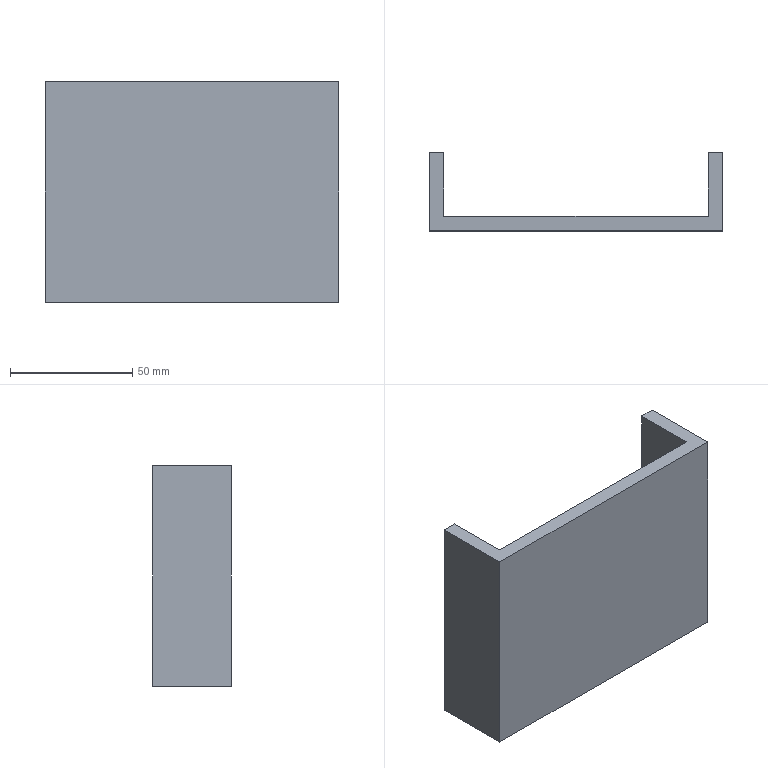Part | SolidWorks | features Extrusion 1 | 1 solid | 10 faces | box 120 x 32 x 90 mm | volume 92880 mm3 | plane 10
STEP:
#1=CARTESIAN_POINT('',(-60.,32.,45.));
#2=VERTEX_POINT('',#1);
#3=CARTESIAN_POINT('',(-60.,0.,45.));
#4=VERTEX_POINT('',#3);
#5=CARTESIAN_POINT('',(-60.,32.,45.));
#6=DIRECTION('',(0.,-1.,0.));
#7=VECTOR('',#6,1000.);
#8=LINE('',#5,#7);
#9=EDGE_CURVE('',#2,#4,#8,.T.);
#10=ORIENTED_EDGE('',*,*,#9,.F.);
#11=CARTESIAN_POINT('',(-60.,32.,-45.));
#12=VERTEX_POINT('',#11);
#13=CARTESIAN_POINT('',(-60.,32.,-45.));
#14=DIRECTION('',(0.,0.,1.));
#15=VECTOR('',#14,1000.);
#16=LINE('',#13,#15);
#17=EDGE_CURVE('',#12,#2,#16,.T.);
#18=ORIENTED_EDGE('',*,*,#17,.F.);
#19=CARTESIAN_POINT('',(-60.,0.,-45.));
#20=VERTEX_POINT('',#19);
#21=CARTESIAN_POINT('',(-60.,32.,-45.));
#22=DIRECTION('',(0.,-1.,0.));
#23=VECTOR('',#22,1000.);
#24=LINE('',#21,#23);
#25=EDGE_CURVE('',#12,#20,#24,.T.);
#26=ORIENTED_EDGE('',*,*,#25,.T.);
#27=CARTESIAN_POINT('',(-60.,0.,-45.));
#28=DIRECTION('',(0.,0.,1.));
#29=VECTOR('',#28,1000.);
#30=LINE('',#27,#29);
#31=EDGE_CURVE('',#20,#4,#30,.T.);
#32=ORIENTED_EDGE('',*,*,#31,.T.);
#33=EDGE_LOOP('',(#10,#18,#26,#32));
#34=FACE_OUTER_BOUND('',#33,.T.);
#35=CARTESIAN_POINT('',(-60.,32.,-45.));
#36=DIRECTION('',(-1.,0.,0.));
#37=DIRECTION('',(0.,0.,1.));
#38=AXIS2_PLACEMENT_3D('',#35,#36,#37);
#39=PLANE('',#38);
#40=ADVANCED_FACE('',(#34),#39,.T.);
#41=CARTESIAN_POINT('',(-54.,32.,45.));
#42=VERTEX_POINT('',#41);
#43=CARTESIAN_POINT('',(-54.,32.,45.));
#44=DIRECTION('',(-1.,0.,0.));
#45=VECTOR('',#44,1000.);
#46=LINE('',#43,#45);
#47=EDGE_CURVE('',#42,#2,#46,.T.);
#48=ORIENTED_EDGE('',*,*,#47,.F.);
#49=CARTESIAN_POINT('',(-54.,32.,-45.));
#50=VERTEX_POINT('',#49);
#51=CARTESIAN_POINT('',(-54.,32.,-45.));
#52=DIRECTION('',(0.,0.,1.));
#53=VECTOR('',#52,1000.);
#54=LINE('',#51,#53);
#55=EDGE_CURVE('',#50,#42,#54,.T.);
#56=ORIENTED_EDGE('',*,*,#55,.F.);
#57=CARTESIAN_POINT('',(-54.,32.,-45.));
#58=DIRECTION('',(-1.,0.,0.));
#59=VECTOR('',#58,1000.);
#60=LINE('',#57,#59);
#61=EDGE_CURVE('',#50,#12,#60,.T.);
#62=ORIENTED_EDGE('',*,*,#61,.T.);
#63=ORIENTED_EDGE('',*,*,#17,.T.);
#64=EDGE_LOOP('',(#48,#56,#62,#63));
#65=FACE_OUTER_BOUND('',#64,.T.);
#66=CARTESIAN_POINT('',(-54.,32.,-45.));
#67=DIRECTION('',(0.,1.,0.));
#68=DIRECTION('',(0.,0.,1.));
#69=AXIS2_PLACEMENT_3D('',#66,#67,#68);
#70=PLANE('',#69);
#71=ADVANCED_FACE('',(#65),#70,.T.);
#72=CARTESIAN_POINT('',(-54.,6.,45.));
#73=VERTEX_POINT('',#72);
#74=CARTESIAN_POINT('',(-54.,6.,45.));
#75=DIRECTION('',(0.,1.,0.));
#76=VECTOR('',#75,1000.);
#77=LINE('',#74,#76);
#78=EDGE_CURVE('',#73,#42,#77,.T.);
#79=ORIENTED_EDGE('',*,*,#78,.F.);
#80=CARTESIAN_POINT('',(-54.,6.,-45.));
#81=VERTEX_POINT('',#80);
#82=CARTESIAN_POINT('',(-54.,6.,-45.));
#83=DIRECTION('',(0.,0.,1.));
#84=VECTOR('',#83,1000.);
#85=LINE('',#82,#84);
#86=EDGE_CURVE('',#81,#73,#85,.T.);
#87=ORIENTED_EDGE('',*,*,#86,.F.);
#88=CARTESIAN_POINT('',(-54.,6.,-45.));
#89=DIRECTION('',(0.,1.,0.));
#90=VECTOR('',#89,1000.);
#91=LINE('',#88,#90);
#92=EDGE_CURVE('',#81,#50,#91,.T.);
#93=ORIENTED_EDGE('',*,*,#92,.T.);
#94=ORIENTED_EDGE('',*,*,#55,.T.);
#95=EDGE_LOOP('',(#79,#87,#93,#94));
#96=FACE_OUTER_BOUND('',#95,.T.);
#97=CARTESIAN_POINT('',(-54.,6.,-45.));
#98=DIRECTION('',(1.,0.,0.));
#99=DIRECTION('',(0.,0.,-1.));
#100=AXIS2_PLACEMENT_3D('',#97,#98,#99);
#101=PLANE('',#100);
#102=ADVANCED_FACE('',(#96),#101,.T.);
#103=CARTESIAN_POINT('',(54.,6.,45.));
#104=VERTEX_POINT('',#103);
#105=CARTESIAN_POINT('',(54.,6.,45.));
#106=DIRECTION('',(-1.,0.,0.));
#107=VECTOR('',#106,1000.);
#108=LINE('',#105,#107);
#109=EDGE_CURVE('',#104,#73,#108,.T.);
#110=ORIENTED_EDGE('',*,*,#109,.F.);
#111=CARTESIAN_POINT('',(54.,6.,-45.));
#112=VERTEX_POINT('',#111);
#113=CARTESIAN_POINT('',(54.,6.,-45.));
#114=DIRECTION('',(0.,0.,1.));
#115=VECTOR('',#114,1000.);
#116=LINE('',#113,#115);
#117=EDGE_CURVE('',#112,#104,#116,.T.);
#118=ORIENTED_EDGE('',*,*,#117,.F.);
#119=CARTESIAN_POINT('',(54.,6.,-45.));
#120=DIRECTION('',(-1.,0.,0.));
#121=VECTOR('',#120,1000.);
#122=LINE('',#119,#121);
#123=EDGE_CURVE('',#112,#81,#122,.T.);
#124=ORIENTED_EDGE('',*,*,#123,.T.);
#125=ORIENTED_EDGE('',*,*,#86,.T.);
#126=EDGE_LOOP('',(#110,#118,#124,#125));
#127=FACE_OUTER_BOUND('',#126,.T.);
#128=CARTESIAN_POINT('',(54.,6.,-45.));
#129=DIRECTION('',(0.,1.,0.));
#130=DIRECTION('',(0.,0.,1.));
#131=AXIS2_PLACEMENT_3D('',#128,#129,#130);
#132=PLANE('',#131);
#133=ADVANCED_FACE('',(#127),#132,.T.);
#134=CARTESIAN_POINT('',(54.,32.,45.));
#135=VERTEX_POINT('',#134);
#136=CARTESIAN_POINT('',(54.,32.,45.));
#137=DIRECTION('',(0.,-1.,0.));
#138=VECTOR('',#137,1000.);
#139=LINE('',#136,#138);
#140=EDGE_CURVE('',#135,#104,#139,.T.);
#141=ORIENTED_EDGE('',*,*,#140,.F.);
#142=CARTESIAN_POINT('',(54.,32.,-45.));
#143=VERTEX_POINT('',#142);
#144=CARTESIAN_POINT('',(54.,32.,-45.));
#145=DIRECTION('',(0.,0.,1.));
#146=VECTOR('',#145,1000.);
#147=LINE('',#144,#146);
#148=EDGE_CURVE('',#143,#135,#147,.T.);
#149=ORIENTED_EDGE('',*,*,#148,.F.);
#150=CARTESIAN_POINT('',(54.,32.,-45.));
#151=DIRECTION('',(0.,-1.,0.));
#152=VECTOR('',#151,1000.);
#153=LINE('',#150,#152);
#154=EDGE_CURVE('',#143,#112,#153,.T.);
#155=ORIENTED_EDGE('',*,*,#154,.T.);
#156=ORIENTED_EDGE('',*,*,#117,.T.);
#157=EDGE_LOOP('',(#141,#149,#155,#156));
#158=FACE_OUTER_BOUND('',#157,.T.);
#159=CARTESIAN_POINT('',(54.,32.,-45.));
#160=DIRECTION('',(-1.,0.,0.));
#161=DIRECTION('',(0.,0.,1.));
#162=AXIS2_PLACEMENT_3D('',#159,#160,#161);
#163=PLANE('',#162);
#164=ADVANCED_FACE('',(#158),#163,.T.);
#165=CARTESIAN_POINT('',(60.,32.,45.));
#166=VERTEX_POINT('',#165);
#167=CARTESIAN_POINT('',(60.,32.,45.));
#168=DIRECTION('',(-1.,0.,0.));
#169=VECTOR('',#168,1000.);
#170=LINE('',#167,#169);
#171=EDGE_CURVE('',#166,#135,#170,.T.);
#172=ORIENTED_EDGE('',*,*,#171,.F.);
#173=CARTESIAN_POINT('',(60.,32.,-45.));
#174=VERTEX_POINT('',#173);
#175=CARTESIAN_POINT('',(60.,32.,-45.));
#176=DIRECTION('',(0.,0.,1.));
#177=VECTOR('',#176,1000.);
#178=LINE('',#175,#177);
#179=EDGE_CURVE('',#174,#166,#178,.T.);
#180=ORIENTED_EDGE('',*,*,#179,.F.);
#181=CARTESIAN_POINT('',(60.,32.,-45.));
#182=DIRECTION('',(-1.,0.,0.));
#183=VECTOR('',#182,1000.);
#184=LINE('',#181,#183);
#185=EDGE_CURVE('',#174,#143,#184,.T.);
#186=ORIENTED_EDGE('',*,*,#185,.T.);
#187=ORIENTED_EDGE('',*,*,#148,.T.);
#188=EDGE_LOOP('',(#172,#180,#186,#187));
#189=FACE_OUTER_BOUND('',#188,.T.);
#190=CARTESIAN_POINT('',(60.,32.,-45.));
#191=DIRECTION('',(0.,1.,0.));
#192=DIRECTION('',(0.,0.,1.));
#193=AXIS2_PLACEMENT_3D('',#190,#191,#192);
#194=PLANE('',#193);
#195=ADVANCED_FACE('',(#189),#194,.T.);
#196=CARTESIAN_POINT('',(60.,0.,45.));
#197=VERTEX_POINT('',#196);
#198=CARTESIAN_POINT('',(60.,0.,45.));
#199=DIRECTION('',(0.,1.,0.));
#200=VECTOR('',#199,1000.);
#201=LINE('',#198,#200);
#202=EDGE_CURVE('',#197,#166,#201,.T.);
#203=ORIENTED_EDGE('',*,*,#202,.F.);
#204=CARTESIAN_POINT('',(60.,0.,-45.));
#205=VERTEX_POINT('',#204);
#206=CARTESIAN_POINT('',(60.,0.,-45.));
#207=DIRECTION('',(0.,0.,1.));
#208=VECTOR('',#207,1000.);
#209=LINE('',#206,#208);
#210=EDGE_CURVE('',#205,#197,#209,.T.);
#211=ORIENTED_EDGE('',*,*,#210,.F.);
#212=CARTESIAN_POINT('',(60.,0.,-45.));
#213=DIRECTION('',(0.,1.,0.));
#214=VECTOR('',#213,1000.);
#215=LINE('',#212,#214);
#216=EDGE_CURVE('',#205,#174,#215,.T.);
#217=ORIENTED_EDGE('',*,*,#216,.T.);
#218=ORIENTED_EDGE('',*,*,#179,.T.);
#219=EDGE_LOOP('',(#203,#211,#217,#218));
#220=FACE_OUTER_BOUND('',#219,.T.);
#221=CARTESIAN_POINT('',(60.,0.,-45.));
#222=DIRECTION('',(1.,0.,0.));
#223=DIRECTION('',(0.,0.,-1.));
#224=AXIS2_PLACEMENT_3D('',#221,#222,#223);
#225=PLANE('',#224);
#226=ADVANCED_FACE('',(#220),#225,.T.);
#227=CARTESIAN_POINT('',(-60.,0.,45.));
#228=DIRECTION('',(1.,0.,0.));
#229=VECTOR('',#228,1000.);
#230=LINE('',#227,#229);
#231=EDGE_CURVE('',#4,#197,#230,.T.);
#232=ORIENTED_EDGE('',*,*,#231,.F.);
#233=ORIENTED_EDGE('',*,*,#31,.F.);
#234=CARTESIAN_POINT('',(-60.,0.,-45.));
#235=DIRECTION('',(1.,0.,0.));
#236=VECTOR('',#235,1000.);
#237=LINE('',#234,#236);
#238=EDGE_CURVE('',#20,#205,#237,.T.);
#239=ORIENTED_EDGE('',*,*,#238,.T.);
#240=ORIENTED_EDGE('',*,*,#210,.T.);
#241=EDGE_LOOP('',(#232,#233,#239,#240));
#242=FACE_OUTER_BOUND('',#241,.T.);
#243=CARTESIAN_POINT('',(-60.,0.,-45.));
#244=DIRECTION('',(0.,-1.,0.));
#245=DIRECTION('',(0.,0.,-1.));
#246=AXIS2_PLACEMENT_3D('',#243,#244,#245);
#247=PLANE('',#246);
#248=ADVANCED_FACE('',(#242),#247,.T.);
#249=ORIENTED_EDGE('',*,*,#25,.F.);
#250=ORIENTED_EDGE('',*,*,#61,.F.);
#251=ORIENTED_EDGE('',*,*,#92,.F.);
#252=ORIENTED_EDGE('',*,*,#123,.F.);
#253=ORIENTED_EDGE('',*,*,#154,.F.);
#254=ORIENTED_EDGE('',*,*,#185,.F.);
#255=ORIENTED_EDGE('',*,*,#216,.F.);
#256=ORIENTED_EDGE('',*,*,#238,.F.);
#257=EDGE_LOOP('',(#249,#250,#251,#252,#253,#254,#255,#256));
#258=FACE_OUTER_BOUND('',#257,.T.);
#259=CARTESIAN_POINT('',(0.,0.,-45.));
#260=DIRECTION('',(0.,0.,1.));
#261=DIRECTION('',(1.,0.,0.));
#262=AXIS2_PLACEMENT_3D('',#259,#260,#261);
#263=PLANE('',#262);
#264=ADVANCED_FACE('',(#258),#263,.F.);
#265=ORIENTED_EDGE('',*,*,#9,.T.);
#266=ORIENTED_EDGE('',*,*,#231,.T.);
#267=ORIENTED_EDGE('',*,*,#202,.T.);
#268=ORIENTED_EDGE('',*,*,#171,.T.);
#269=ORIENTED_EDGE('',*,*,#140,.T.);
#270=ORIENTED_EDGE('',*,*,#109,.T.);
#271=ORIENTED_EDGE('',*,*,#78,.T.);
#272=ORIENTED_EDGE('',*,*,#47,.T.);
#273=EDGE_LOOP('',(#265,#266,#267,#268,#269,#270,#271,#272));
#274=FACE_OUTER_BOUND('',#273,.T.);
#275=CARTESIAN_POINT('',(0.,0.,45.));
#276=DIRECTION('',(0.,0.,1.));
#277=DIRECTION('',(1.,0.,0.));
#278=AXIS2_PLACEMENT_3D('',#275,#276,#277);
#279=PLANE('',#278);
#280=ADVANCED_FACE('',(#274),#279,.T.);
#281=CLOSED_SHELL('',(#40,#71,#102,#133,#164,#195,#226,#248,#264,#280));
#282=MANIFOLD_SOLID_BREP('',#281);
#283=CARTESIAN_POINT('',(0.,0.,0.));
#284=DIRECTION('',(0.,0.,1.));
#285=DIRECTION('',(1.,0.,0.));
#286=AXIS2_PLACEMENT_3D('',#283,#284,#285);
#287=(LENGTH_UNIT()NAMED_UNIT(*)SI_UNIT(.MILLI.,.METRE.));
#288=UNCERTAINTY_MEASURE_WITH_UNIT(LENGTH_MEASURE(0.00001),#287,'','');
#289=(NAMED_UNIT(*)PLANE_ANGLE_UNIT()SI_UNIT($,.RADIAN.));
#290=(NAMED_UNIT(*)SI_UNIT($,.STERADIAN.)SOLID_ANGLE_UNIT());
#291=(GEOMETRIC_REPRESENTATION_CONTEXT(3)GLOBAL_UNCERTAINTY_ASSIGNED_CONTEXT((#288))GLOBAL_UNIT_ASSIGNED_CONTEXT((#287,#289,#290))REPRESENTATION_CONTEXT('',''));
#292=ADVANCED_BREP_SHAPE_REPRESENTATION('',(#282,#286),#291);